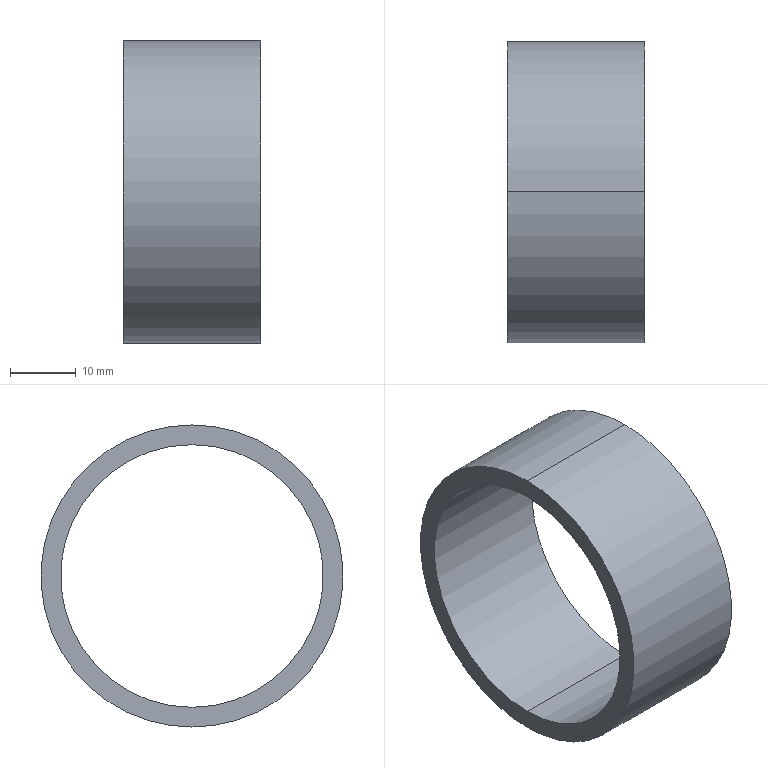Part | SolidWorks | features Extrusion 1 | 1 solid | 6 faces | box 21 x 46 x 46 mm | volume 8511 mm3 | cylinder 4 | plane 2 | commonest cylinder face diameters 40 x2 46 x2
STEP:
#1=CARTESIAN_POINT('',(21.,0.,20.));
#2=VERTEX_POINT('',#1);
#3=CARTESIAN_POINT('',(21.,0.,-20.));
#4=VERTEX_POINT('',#3);
#5=CARTESIAN_POINT('',(21.,0.,0.));
#6=DIRECTION('',(1.,0.,0.));
#7=DIRECTION('',(0.,0.,-1.));
#8=AXIS2_PLACEMENT_3D('',#5,#6,#7);
#9=CIRCLE('',#8,20.);
#10=EDGE_CURVE('',#2,#4,#9,.T.);
#11=ORIENTED_EDGE('',*,*,#10,.T.);
#12=CARTESIAN_POINT('',(0.,0.,-20.));
#13=VERTEX_POINT('',#12);
#14=CARTESIAN_POINT('',(21.,0.,-20.));
#15=DIRECTION('',(-1.,0.,0.));
#16=VECTOR('',#15,1000.);
#17=LINE('',#14,#16);
#18=EDGE_CURVE('',#4,#13,#17,.T.);
#19=ORIENTED_EDGE('',*,*,#18,.T.);
#20=CARTESIAN_POINT('',(0.,0.,20.));
#21=VERTEX_POINT('',#20);
#22=CARTESIAN_POINT('',(0.,0.,0.));
#23=DIRECTION('',(1.,0.,0.));
#24=DIRECTION('',(0.,0.,-1.));
#25=AXIS2_PLACEMENT_3D('',#22,#23,#24);
#26=CIRCLE('',#25,20.);
#27=EDGE_CURVE('',#21,#13,#26,.T.);
#28=ORIENTED_EDGE('',*,*,#27,.F.);
#29=CARTESIAN_POINT('',(21.,0.,20.));
#30=DIRECTION('',(-1.,0.,0.));
#31=VECTOR('',#30,1000.);
#32=LINE('',#29,#31);
#33=EDGE_CURVE('',#2,#21,#32,.T.);
#34=ORIENTED_EDGE('',*,*,#33,.F.);
#35=EDGE_LOOP('',(#11,#19,#28,#34));
#36=FACE_OUTER_BOUND('',#35,.T.);
#37=CARTESIAN_POINT('',(21.,0.,0.));
#38=DIRECTION('',(-1.,0.,0.));
#39=DIRECTION('',(0.,0.,1.));
#40=AXIS2_PLACEMENT_3D('',#37,#38,#39);
#41=CYLINDRICAL_SURFACE('',#40,20.);
#42=ADVANCED_FACE('',(#36),#41,.F.);
#43=CARTESIAN_POINT('',(21.,0.,-23.));
#44=VERTEX_POINT('',#43);
#45=CARTESIAN_POINT('',(21.,0.,23.));
#46=VERTEX_POINT('',#45);
#47=CARTESIAN_POINT('',(21.,0.,0.));
#48=DIRECTION('',(1.,0.,0.));
#49=DIRECTION('',(0.,0.,-1.));
#50=AXIS2_PLACEMENT_3D('',#47,#48,#49);
#51=CIRCLE('',#50,23.);
#52=EDGE_CURVE('',#44,#46,#51,.T.);
#53=ORIENTED_EDGE('',*,*,#52,.F.);
#54=CARTESIAN_POINT('',(0.,0.,-23.));
#55=VERTEX_POINT('',#54);
#56=CARTESIAN_POINT('',(21.,0.,-23.));
#57=DIRECTION('',(-1.,0.,0.));
#58=VECTOR('',#57,1000.);
#59=LINE('',#56,#58);
#60=EDGE_CURVE('',#44,#55,#59,.T.);
#61=ORIENTED_EDGE('',*,*,#60,.T.);
#62=CARTESIAN_POINT('',(0.,0.,23.));
#63=VERTEX_POINT('',#62);
#64=CARTESIAN_POINT('',(0.,0.,0.));
#65=DIRECTION('',(1.,0.,0.));
#66=DIRECTION('',(0.,0.,-1.));
#67=AXIS2_PLACEMENT_3D('',#64,#65,#66);
#68=CIRCLE('',#67,23.);
#69=EDGE_CURVE('',#55,#63,#68,.T.);
#70=ORIENTED_EDGE('',*,*,#69,.T.);
#71=CARTESIAN_POINT('',(21.,0.,23.));
#72=DIRECTION('',(-1.,0.,0.));
#73=VECTOR('',#72,1000.);
#74=LINE('',#71,#73);
#75=EDGE_CURVE('',#46,#63,#74,.T.);
#76=ORIENTED_EDGE('',*,*,#75,.F.);
#77=EDGE_LOOP('',(#53,#61,#70,#76));
#78=FACE_OUTER_BOUND('',#77,.T.);
#79=CARTESIAN_POINT('',(21.,0.,0.));
#80=DIRECTION('',(-1.,0.,0.));
#81=DIRECTION('',(0.,0.,1.));
#82=AXIS2_PLACEMENT_3D('',#79,#80,#81);
#83=CYLINDRICAL_SURFACE('',#82,23.);
#84=ADVANCED_FACE('',(#78),#83,.T.);
#85=CARTESIAN_POINT('',(21.,0.,0.));
#86=DIRECTION('',(1.,0.,0.));
#87=DIRECTION('',(0.,0.,-1.));
#88=AXIS2_PLACEMENT_3D('',#85,#86,#87);
#89=CIRCLE('',#88,23.);
#90=EDGE_CURVE('',#46,#44,#89,.T.);
#91=ORIENTED_EDGE('',*,*,#90,.T.);
#92=ORIENTED_EDGE('',*,*,#52,.T.);
#93=EDGE_LOOP('',(#91,#92));
#94=FACE_OUTER_BOUND('',#93,.T.);
#95=ORIENTED_EDGE('',*,*,#10,.F.);
#96=CARTESIAN_POINT('',(21.,0.,0.));
#97=DIRECTION('',(1.,0.,0.));
#98=DIRECTION('',(0.,0.,-1.));
#99=AXIS2_PLACEMENT_3D('',#96,#97,#98);
#100=CIRCLE('',#99,20.);
#101=EDGE_CURVE('',#4,#2,#100,.T.);
#102=ORIENTED_EDGE('',*,*,#101,.F.);
#103=EDGE_LOOP('',(#95,#102));
#104=FACE_BOUND('',#103,.T.);
#105=CARTESIAN_POINT('',(21.,0.,0.));
#106=DIRECTION('',(1.,0.,0.));
#107=DIRECTION('',(0.,0.,-1.));
#108=AXIS2_PLACEMENT_3D('',#105,#106,#107);
#109=PLANE('',#108);
#110=ADVANCED_FACE('',(#94,#104),#109,.T.);
#111=CARTESIAN_POINT('',(0.,0.,0.));
#112=DIRECTION('',(1.,0.,0.));
#113=DIRECTION('',(0.,0.,-1.));
#114=AXIS2_PLACEMENT_3D('',#111,#112,#113);
#115=CIRCLE('',#114,23.);
#116=EDGE_CURVE('',#63,#55,#115,.T.);
#117=ORIENTED_EDGE('',*,*,#116,.F.);
#118=ORIENTED_EDGE('',*,*,#69,.F.);
#119=EDGE_LOOP('',(#117,#118));
#120=FACE_OUTER_BOUND('',#119,.T.);
#121=ORIENTED_EDGE('',*,*,#27,.T.);
#122=CARTESIAN_POINT('',(0.,0.,0.));
#123=DIRECTION('',(1.,0.,0.));
#124=DIRECTION('',(0.,0.,-1.));
#125=AXIS2_PLACEMENT_3D('',#122,#123,#124);
#126=CIRCLE('',#125,20.);
#127=EDGE_CURVE('',#13,#21,#126,.T.);
#128=ORIENTED_EDGE('',*,*,#127,.T.);
#129=EDGE_LOOP('',(#121,#128));
#130=FACE_BOUND('',#129,.T.);
#131=CARTESIAN_POINT('',(0.,0.,0.));
#132=DIRECTION('',(1.,0.,0.));
#133=DIRECTION('',(0.,0.,-1.));
#134=AXIS2_PLACEMENT_3D('',#131,#132,#133);
#135=PLANE('',#134);
#136=ADVANCED_FACE('',(#120,#130),#135,.F.);
#137=ORIENTED_EDGE('',*,*,#60,.F.);
#138=ORIENTED_EDGE('',*,*,#90,.F.);
#139=ORIENTED_EDGE('',*,*,#75,.T.);
#140=ORIENTED_EDGE('',*,*,#116,.T.);
#141=EDGE_LOOP('',(#137,#138,#139,#140));
#142=FACE_OUTER_BOUND('',#141,.T.);
#143=CARTESIAN_POINT('',(21.,0.,0.));
#144=DIRECTION('',(-1.,0.,0.));
#145=DIRECTION('',(0.,0.,1.));
#146=AXIS2_PLACEMENT_3D('',#143,#144,#145);
#147=CYLINDRICAL_SURFACE('',#146,23.);
#148=ADVANCED_FACE('',(#142),#147,.T.);
#149=ORIENTED_EDGE('',*,*,#18,.F.);
#150=ORIENTED_EDGE('',*,*,#101,.T.);
#151=ORIENTED_EDGE('',*,*,#33,.T.);
#152=ORIENTED_EDGE('',*,*,#127,.F.);
#153=EDGE_LOOP('',(#149,#150,#151,#152));
#154=FACE_OUTER_BOUND('',#153,.T.);
#155=CARTESIAN_POINT('',(21.,0.,0.));
#156=DIRECTION('',(-1.,0.,0.));
#157=DIRECTION('',(0.,0.,1.));
#158=AXIS2_PLACEMENT_3D('',#155,#156,#157);
#159=CYLINDRICAL_SURFACE('',#158,20.);
#160=ADVANCED_FACE('',(#154),#159,.F.);
#161=CLOSED_SHELL('',(#42,#84,#110,#136,#148,#160));
#162=MANIFOLD_SOLID_BREP('',#161);
#163=CARTESIAN_POINT('',(0.,0.,0.));
#164=DIRECTION('',(0.,0.,1.));
#165=DIRECTION('',(1.,0.,0.));
#166=AXIS2_PLACEMENT_3D('',#163,#164,#165);
#167=(LENGTH_UNIT()NAMED_UNIT(*)SI_UNIT(.MILLI.,.METRE.));
#168=UNCERTAINTY_MEASURE_WITH_UNIT(LENGTH_MEASURE(0.00001),#167,'','');
#169=(NAMED_UNIT(*)PLANE_ANGLE_UNIT()SI_UNIT($,.RADIAN.));
#170=(NAMED_UNIT(*)SI_UNIT($,.STERADIAN.)SOLID_ANGLE_UNIT());
#171=(GEOMETRIC_REPRESENTATION_CONTEXT(3)GLOBAL_UNCERTAINTY_ASSIGNED_CONTEXT((#168))GLOBAL_UNIT_ASSIGNED_CONTEXT((#167,#169,#170))REPRESENTATION_CONTEXT('',''));
#172=ADVANCED_BREP_SHAPE_REPRESENTATION('',(#162,#166),#171);